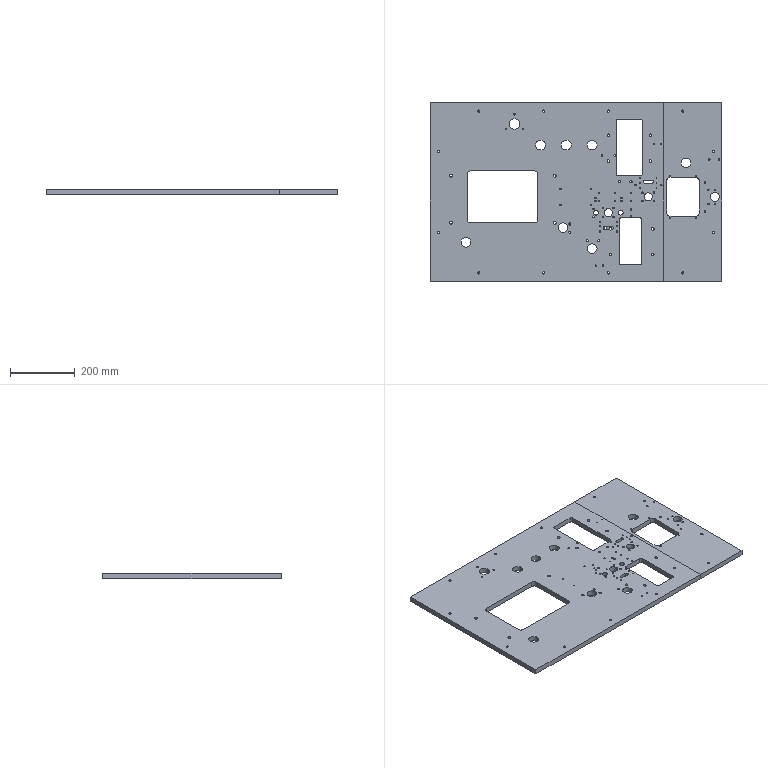Part | STEP file | base plate | 2 solids | 272 faces | box 900 x 550 x 16 mm | volume 6619643 mm3 | cylinder 231 | plane 41 | commonest cylinder face diameters 4.2 x65 5 x54 6.8 x24 8.5 x16 30 x14 7 x12